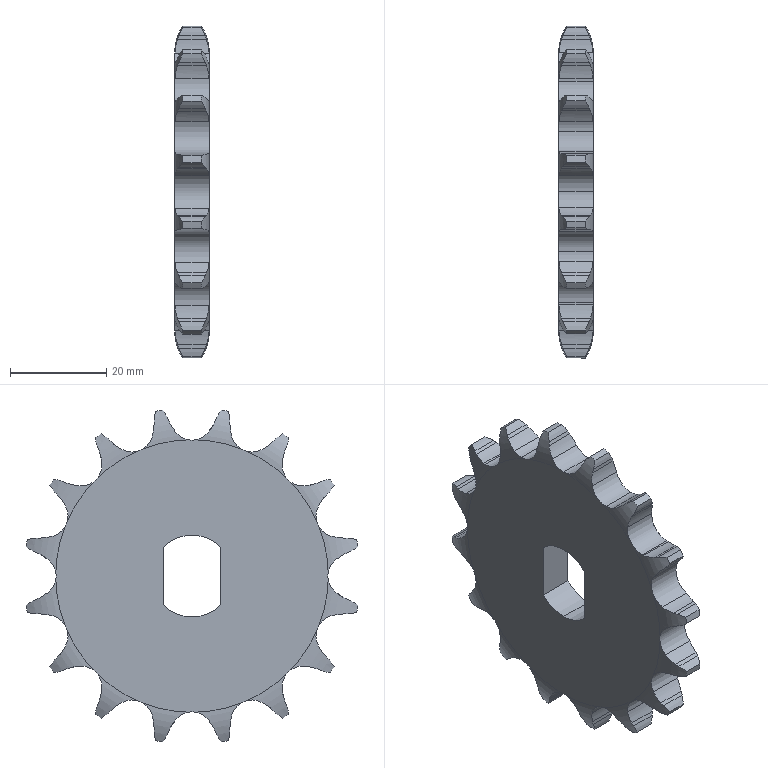Part | SolidWorks | features BaseBody 1 | 1 solid | 172 faces | box 7.222 x 68.92 x 68.92 mm | volume 19661 mm3 | cylinder 104 | plane 36 | torus 32 | commonest cylinder face diameters 12.473 x32 22.269 x32 8.653 x21 70 x16 17 x3